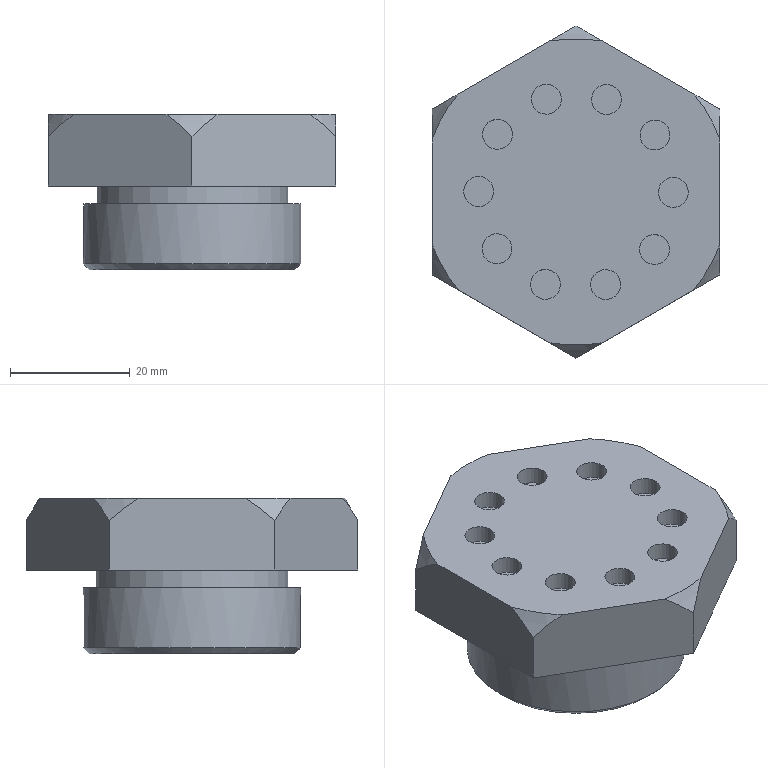Part | NX | features CYLINDER 5, DATUM_CSYS 3, EXTRUDE 3, CHAMFER 2, SKETCH 2, INTERSECT 1, SYMBOLIC_THREAD 1 | 1 solid | 45 faces | volume 32370 mm3 | plane 23 | cylinder 15 | cone 7 | commonest cylinder face diameters 5 x10 6 x1 10 x1 25 x1 32 x1 36.292 x1